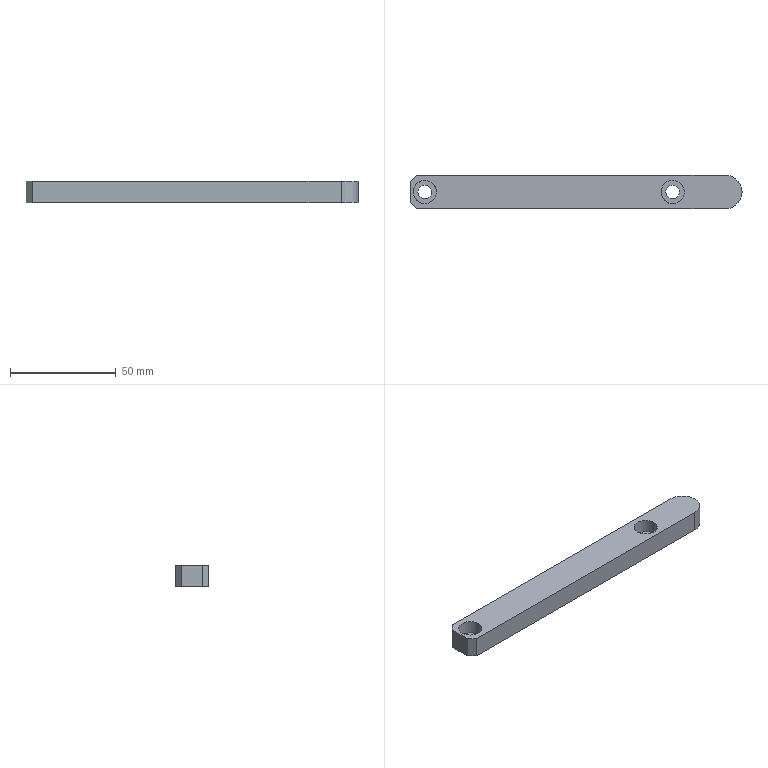Part | STEP file | 1_id1486_x_t | 1 solid | 27 faces | box 156.936 x 16 x 10 mm | volume 21479 mm3 | cylinder 15 | plane 12 | commonest cylinder face diameters 12 x6 6.5 x4 11 x4 16 x1